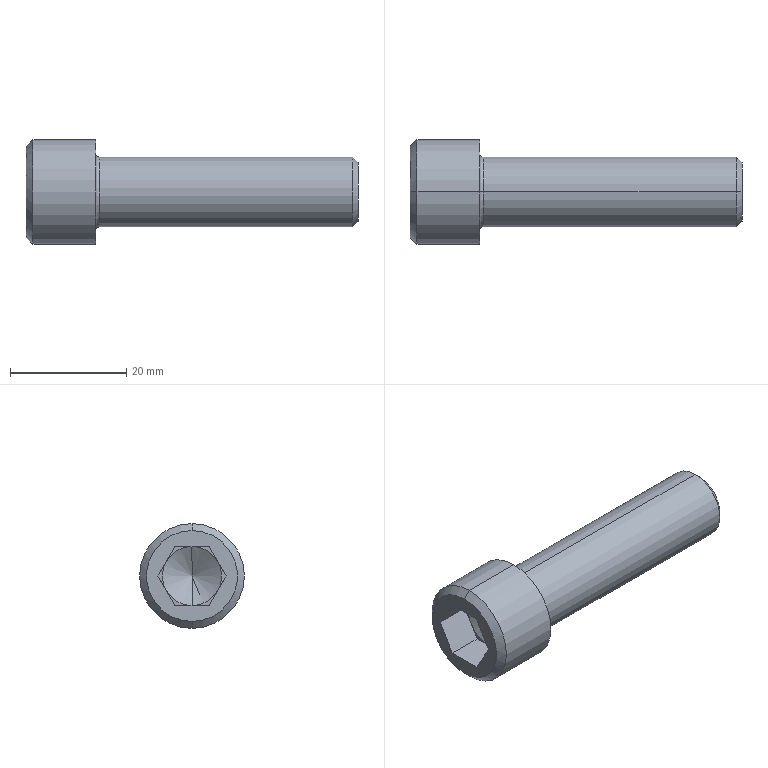Part | STEP file | socket head cap screw_am_B18.3.1M - 12 x 1.75 x 45 Hex SHCS -- 45NHX | 1 solid | 27 faces | box 57 x 18 x 18 mm | volume 7481 mm3 | plane 15 | cone 6 | cylinder 4 | torus 2 | commonest cylinder face diameters 12 x2 18 x2